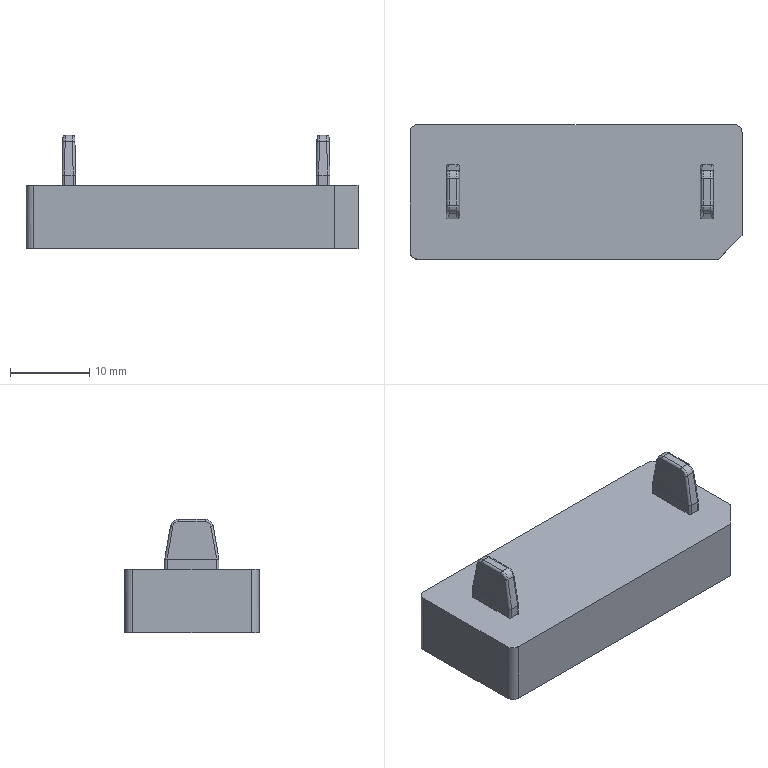NC program | PowerMill | posted by the shop | part box 42 x 17 x 14.346 mm
Lines 3506 to 4334 of 86217:
( TOOL ID   D10_1_1 )
( TOOL DIA. 10. TIP RAD 0 LENGTH 69.52 )
( Z = -.274 )
T3 M6
T4
G91 G28 Z0
G0 G90 G54
M08
S8500 M3
X0 Y0 M8
G43 Z11.796 H3
X-11.537 Y-11.817
Z.926
G1 Z-.274 F360
X-13.342 Y-6.86 F600
X-13.849 Y7.05
X-14.067 Y7.097
X-14.384 Y7.153
X-14.7 Y7.182
X-15.017 Y7.195
X-15.333 Y7.194
X-15.649 Y7.186
X-16.282 Y7.179
X-16.598 Y7.157
X-16.914 Y7.115
X-17.231 Y7.053
X-17.547 Y6.97
X-17.819 Y6.883
X-17.313 Y-7.01
G0 Z3.996
G1 X21.398 Y-11.505 F10000
G0 Z.926
G1 Z-.274 F360
X19.185 Y-6.717 F600
X17.985 Y7.118
X17.863 Y7.14
X17.547 Y7.175
X17.23 Y7.195
X16.914 Y7.199
X16.598 Y7.185
X15.965 Y7.184
X15.649 Y7.164
X15.332 Y7.128
X15.016 Y7.072
X14.699 Y6.996
X14.383 Y6.897
X14.067 Y6.779
X13.974 Y6.738
X15.172 Y-7.076
G0 Z11.796
X0 Y0
Z9.796
X31.66 Y.061
Z-5.35
G1 Z-6.55 F360
X26.385 F600
X22.805
Y-3.109
X22.798 Y-3.392
X22.769 Y-3.737
X22.733 Y-4.009
X22.683 Y-4.278
X22.62 Y-4.545
X22.524 Y-4.869
X22.441 Y-5.109
X22.346 Y-5.346
X22.241 Y-5.578
X22.124 Y-5.805
G2 X21.841 Y-6.277 I-5.278 J2.842
X21.512 Y-6.718 I-5.134 J3.488
G1 X21.346 Y-6.913
G2 X20.985 Y-7.279 I-4.426 J3.999
X20.554 Y-7.641 I-4.73 J5.201
X19.7 Y-8.174 I-3.44 J4.554
G1 X19.414 Y-8.312
X19.173 Y-8.411
X18.868 Y-8.518
X18.598 Y-8.599
X18.325 Y-8.666
X18.048 Y-8.718
X17.769 Y-8.756
G2 X17.124 Y-8.794 I-.663 J5.709
G1 X15.841 Y-8.791
X15.616 Y-8.778
X15.391 Y-8.756
X15.112 Y-8.718
X14.835 Y-8.666
X14.562 Y-8.599
G2 X13.987 Y-8.411 I1.929 J6.87
G1 X13.746 Y-8.312
G2 X13.232 Y-8.052 I2.536 J5.659
G1 X13.017 Y-7.925
G2 X12.591 Y-7.629 I3.181 J5.035
G1 X12.41 Y-7.485
G2 X11.99 Y-7.1 I3.923 J4.714
X11.319 Y-6.277 I4.33 J4.216
G1 X11.186 Y-6.068
X11.036 Y-5.805
X10.919 Y-5.578
G2 X10.617 Y-4.808 I5.201 J2.49
G1 X10.54 Y-4.545
X10.477 Y-4.278
X10.427 Y-4.009
X10.391 Y-3.737
X10.362 Y-3.392
X10.355 Y-3.109
Y3.148
X10.362 Y3.431
X10.391 Y3.776
X10.427 Y4.048
X10.477 Y4.318
X10.54 Y4.584
X10.636 Y4.908
X10.719 Y5.149
X10.814 Y5.385
X10.919 Y5.617
X11.036 Y5.844
G2 X11.319 Y6.316 I5.259 J-2.831
X11.648 Y6.757 I5.132 J-3.486
G1 X11.814 Y6.952
G2 X12.175 Y7.318 I4.415 J-3.988
X12.606 Y7.68 I4.7 J-5.165
X13.017 Y7.964 I3.646 J-4.838
G1 X13.28 Y8.118
X13.511 Y8.24
X13.746 Y8.351
X14.016 Y8.461
X14.233 Y8.538
G2 X14.835 Y8.705 I1.983 J-5.972
G1 X15.112 Y8.757
X15.391 Y8.795
G2 X16.036 Y8.834 I.667 J-5.782
G1 X17.233 Y8.832
G2 X17.9 Y8.777 I-.091 J-5.246
G1 X18.048 Y8.757
G2 X18.598 Y8.638 I-1.065 J-6.25
X19.173 Y8.45 I-1.914 J-6.822
X20.093 Y7.993 I-2.078 J-5.341
G1 X20.257 Y7.89
X20.554 Y7.68
X20.792 Y7.488
X20.985 Y7.318
X21.17 Y7.14
G2 X21.974 Y6.108 I-4.196 J-4.1
G1 X22.097 Y5.893
G2 X22.346 Y5.385 I-5.508 J-3.016
G1 X22.441 Y5.149
X22.543 Y4.848
X22.62 Y4.584
X22.683 Y4.318
X22.733 Y4.048
X22.769 Y3.776
X22.798 Y3.431
X22.805 Y3.148
Y.061
X26.385
G0 Z2.856
G1 X-31.66 Y.02 F10000
G0 Z-5.35
G1 Z-6.55 F360
X-26.385 F600
X-21.805
Y3.148
X-21.798 Y3.431
X-21.769 Y3.776
X-21.733 Y4.048
X-21.683 Y4.318
X-21.62 Y4.584
X-21.51 Y4.951
X-21.441 Y5.149
X-21.346 Y5.385
X-21.241 Y5.617
G2 X-20.841 Y6.316 I5.578 J-2.725
G1 X-20.699 Y6.518
X-20.512 Y6.757
X-20.346 Y6.952
X-20.17 Y7.14
G2 X-19.717 Y7.549 I4.101 J-4.072
G1 X-19.554 Y7.68
G2 X-18.946 Y8.08 I3.381 J-4.47
X-18.173 Y8.45 I2.795 J-4.851
X-17.598 Y8.638 I2.5 J-6.67
X-17.048 Y8.757 I1.632 J-6.207
G1 X-16.769 Y8.795
G2 X-16.124 Y8.834 I.668 J-5.798
G1 X-14.947 Y8.832
G2 X-14.271 Y8.779 I-.068 J-5.2
G1 X-14.112 Y8.757
X-13.835 Y8.705
G2 X-13.122 Y8.499 I-1.254 J-5.662
X-12.42 Y8.192 I-1.656 J-4.761
X-11.549 Y7.635 I-2.474 J-4.822
G1 X-11.359 Y7.48
X-11.175 Y7.318
X-10.99 Y7.14
X-10.814 Y6.952
G2 X-10.461 Y6.518 I-5.166 J-4.566
X-10.036 Y5.844 I-4.569 J-3.352
G1 X-9.919 Y5.617
G2 X-9.719 Y5.149 I-5.583 J-2.662
G1 X-9.617 Y4.848
X-9.54 Y4.584
X-9.477 Y4.318
X-9.427 Y4.048
X-9.385 Y3.713
X-9.362 Y3.431
X-9.355 Y3.148
Y.487
X.465 Y.636
X.514 Y-2.554
G2 X.474 Y-3.952 I-16.134 J-.244
G1 X.469 Y-4.025
G3 X.52 Y-4.08 I.051 J-.004
G1 X.54
G3 X.592 Y-4.025 I0 J.052
G1 X.57 Y-3.53
X.478 Y2.325
G2 X.529 Y3.956 I17.263 J.27
G1 X.535 Y4.032
G3 X.485 Y4.087 I-.051 J.004
G1 X.461
G3 X.408 Y4.031 I0 J-.053
G1 X.417 Y3.826
X.465 Y.636
X-4.521 Y.56
X-4.56 Y3.429
X-4.573 Y3.696
G3 X-5.417 Y7.309 I-10.448 J-.535
G1 X-5.709 Y7.986
G2 X-4.991 Y9.078 I.718 J.31
G1 X5.994 Y9.079
G2 X6.705 Y7.974 I0 J-.781
G1 X6.571 Y7.68
G3 X5.469 Y2.408 I11.158 J-5.085
G1 X5.558 Y-3.337
G3 X5.97 Y-6.021 I10.686 J.264
G1 X6.101 Y-6.446
G3 X6.445 Y-7.339 I9.337 J3.09
G1 X6.532 Y-7.535
X6.737 Y-7.95
G2 X6.047 Y-9.065 I-.69 J-.344
G1 X-5.017 Y-9.079
G2 X-5.725 Y-7.971 I-.001 J.78
G1 X-5.592 Y-7.683
X-5.332 Y-7.082
X-5.268 Y-6.921
G3 X-4.477 Y-2.647 I-10.334 J4.122
G1 X-4.521 Y.56
X-9.355 Y.487
Y-3.109
X-9.362 Y-3.392
G2 X-9.427 Y-4.009 I-7.113 J.434
G1 X-9.477 Y-4.278
G2 X-9.814 Y-5.346 I-5.909 J1.278
G1 X-9.919 Y-5.578
X-10.063 Y-5.854
X-10.186 Y-6.068
X-10.319 Y-6.277
X-10.461 Y-6.479
G2 X-10.99 Y-7.1 I-4.994 J3.717
G1 X-11.175 Y-7.279
X-11.41 Y-7.485
X-11.606 Y-7.641
X-11.808 Y-7.787
X-12.017 Y-7.925
X-12.227 Y-8.049
X-12.511 Y-8.201
G2 X-12.987 Y-8.411 I-2.772 J5.65
G1 X-13.292 Y-8.518
X-13.562 Y-8.599
X-13.835 Y-8.666
X-14.112 Y-8.718
X-14.391 Y-8.756
G2 X-15.036 Y-8.794 I-.659 J5.646
G1 X-16.124
X-16.319 Y-8.791
G2 X-17.325 Y-8.666 I.251 J6.13
X-18.414 Y-8.312 I1.32 J5.917
X-19.352 Y-7.787 I2.453 J5.49
X-19.792 Y-7.449 I3.506 J5.014
G1 X-19.985 Y-7.279
X-20.17 Y-7.1
X-20.346 Y-6.913
G2 X-20.699 Y-6.479 I5.161 J4.562
X-21.124 Y-5.805 I4.594 J3.368
G1 X-21.241 Y-5.578
G2 X-21.441 Y-5.109 I5.678 J2.703
G1 X-21.543 Y-4.808
X-21.62 Y-4.545
X-21.683 Y-4.278
X-21.733 Y-4.009
X-21.769 Y-3.737
G2 X-21.805 Y-3.109 I6.227 J.676
G1 Y.02
X-26.385
G0 Z9.796
X0 Y0
X26.008 Y-14.747
Z-13.25
G1 Z-14.45 F360
G3 X22.473 Y-11.211 I-1.768 J1.768 F600
G1 X21.614 Y-12.07
X21.613 Y-12.071
X21.395 Y-12.279
X21.394 Y-12.28
X21.392 Y-12.281
X21.267 Y-12.39
X21.266 Y-12.391
X21.265 Y-12.392
X21.074 Y-12.545
X21.072 Y-12.546
X21.07 Y-12.547
X20.842 Y-12.711
X20.84 Y-12.712
X20.839 Y-12.713
X20.752 Y-12.77
X20.75 Y-12.771
X20.748 Y-12.772
X20.432 Y-12.96
X20.43 Y-12.961
X20.429 Y-12.962
X20.293 Y-13.033
X20.292
X20.291 Y-13.034
X20.11 Y-13.121
X20.108 Y-13.122
X20.106 Y-13.123
X19.79 Y-13.254
X19.787 Y-13.255
X19.785 Y-13.256
X19.499 Y-13.354
X19.496 Y-13.355
X19.494
X19.148 Y-13.449
X19.145
X19.142 Y-13.45
X18.826 Y-13.512
X18.824 Y-13.513
X18.821
X18.505 Y-13.555
X18.502
X18.5
X18.184 Y-13.577
X18.181
X18.179
X17.863 Y-13.58
X17.862
X-20.075 Y-13.579
X-20.077
X-20.078
X-20.394 Y-13.567
X-20.397
X-20.399
X-20.715 Y-13.538
X-20.717 Y-13.537
X-20.719
X-21.035 Y-13.491
X-21.037
X-21.039 Y-13.49
X-21.356 Y-13.427
X-21.358 Y-13.426
X-21.36
X-21.636 Y-13.356
X-21.638 Y-13.355
X-21.64 Y-13.354
X-21.996 Y-13.243
X-21.998 Y-13.242
X-22.001 Y-13.241
X-22.317 Y-13.121
X-22.319 Y-13.12
X-22.321
X-22.637 Y-12.978
X-22.639 Y-12.977
X-22.641 Y-12.976
X-22.957 Y-12.812
X-22.959 Y-12.811
X-22.961 Y-12.81
X-23.125 Y-12.715
X-23.127 Y-12.714
X-23.128
X-23.279 Y-12.62
X-23.28 Y-12.619
X-23.282 Y-12.618
X-23.598 Y-12.401
X-23.6 Y-12.399
X-23.602 Y-12.398
X-23.919 Y-12.149
X-23.92 Y-12.148
X-23.921 Y-12.147
X-24.005 Y-12.074
X-24.006 Y-12.073
X-24.008 Y-12.072
X-24.239 Y-11.858
X-24.241 Y-11.857
X-24.242 Y-11.856
X-24.344 Y-11.754
X-24.345 Y-11.753
X-24.346 Y-11.752
X-24.56 Y-11.522
X-24.561 Y-11.52
X-24.562 Y-11.519
X-24.636 Y-11.433
X-24.637 Y-11.432
Y-11.431
X-24.88 Y-11.126
X-24.882 Y-11.124
X-24.883 Y-11.122
X-25.11 Y-10.794
X-25.111 Y-10.793
X-25.112 Y-10.791
X-25.201 Y-10.648
X-25.202 Y-10.647
X-25.203 Y-10.646
X-25.303 Y-10.473
X-25.304 Y-10.471
X-25.305 Y-10.47
X-25.47 Y-10.154
X-25.471 Y-10.152
X-25.472 Y-10.149
X-25.614 Y-9.833
X-25.615 Y-9.831
X-25.616 Y-9.829
X-25.737 Y-9.513
X-25.738 Y-9.511
X-25.739 Y-9.509
X-25.84 Y-9.193
Y-9.19
X-25.841 Y-9.188
X-25.923 Y-8.872
X-25.924 Y-8.87
Y-8.868
X-25.988 Y-8.552
Y-8.55
Y-8.548
X-26.036 Y-8.232
Y-8.229
Y-8.227
X-26.065 Y-7.911
Y-7.909
X-26.066 Y-7.907
X-26.079 Y-7.591
Y-7.589
Y-7.587
Y7.587
Y7.589
Y7.591
X-26.066 Y7.907
Y7.909
Y7.911
X-26.036 Y8.227
Y8.229
Y8.231
X-25.989 Y8.548
Y8.55
X-25.988 Y8.552
X-25.924 Y8.868
Y8.87
X-25.923 Y8.872
X-25.843 Y9.179
Y9.182
X-25.842 Y9.184
X-25.738 Y9.509
Y9.511
X-25.737 Y9.513
X-25.616 Y9.829
X-25.615 Y9.831
X-25.614 Y9.833
X-25.472 Y10.149
X-25.471 Y10.152
X-25.47 Y10.154
X-25.305 Y10.47
X-25.304 Y10.471
X-25.303 Y10.473
X-25.203 Y10.646
X-25.202 Y10.647
X-25.201 Y10.648
X-25.112 Y10.791
X-25.111 Y10.793
X-25.11 Y10.794
X-24.892 Y11.111
X-24.89 Y11.113
X-24.889 Y11.115
X-24.638 Y11.431
X-24.637 Y11.432
X-24.636 Y11.434
X-24.562 Y11.519
X-24.561 Y11.521
X-24.56 Y11.522
X-24.346 Y11.752
X-24.345 Y11.753
X-24.344 Y11.754
X-24.242 Y11.856
X-24.241 Y11.857
X-24.239 Y11.858
X-24.007 Y12.072
X-24.006 Y12.073
X-24.005 Y12.074
X-23.921 Y12.146
X-23.92 Y12.147
X-23.919 Y12.148
X-23.61 Y12.392
X-23.608 Y12.394
X-23.605 Y12.396
X-23.282 Y12.618
X-23.28 Y12.619
X-23.279 Y12.62
X-23.128 Y12.714
X-23.127
X-23.125 Y12.715
X-22.961 Y12.81
X-22.959 Y12.811
X-22.957 Y12.812
X-22.641 Y12.976
X-22.639 Y12.977
X-22.637 Y12.978
X-22.321 Y13.12
X-22.319
X-22.317 Y13.121
X-22.001 Y13.241
X-21.998 Y13.242
X-21.996 Y13.243
X-21.68 Y13.343
X-21.678 Y13.344
X-21.676
X-21.36 Y13.426
X-21.358
X-21.355 Y13.427
X-21.039 Y13.49
X-21.037
X-21.035
X-20.719 Y13.537
X-20.717
X-20.715 Y13.538
X-20.399 Y13.566
X-20.397
X-20.395
X-20.079 Y13.579
X-20.077
X-20.075
X-.316
X20.075
X20.077
X20.078
X20.394 Y13.567
X20.397
X20.399
X20.715 Y13.538
X20.717 Y13.537
X20.719
X21.035 Y13.491
X21.037
X21.039 Y13.49
X21.356 Y13.427
X21.358 Y13.426
X21.36
X21.636 Y13.356
X21.638 Y13.355
X21.64 Y13.354
X21.996 Y13.243
X21.998 Y13.242
X22.001 Y13.241
X22.317 Y13.121
X22.319 Y13.12
X22.321
X22.637 Y12.978
X22.639 Y12.977
X22.641 Y12.976
X22.957 Y12.812
X22.959 Y12.811
X22.961 Y12.81
X23.125 Y12.715
X23.127 Y12.714
X23.128
X23.279 Y12.62
X23.28 Y12.619
X23.282 Y12.618
X23.598 Y12.401
X23.6 Y12.399
X23.602 Y12.398
X23.919 Y12.149
X23.92 Y12.148
X23.921 Y12.147
X24.005 Y12.074
X24.006 Y12.073
X24.008 Y12.072
X24.239 Y11.858
X24.241 Y11.857
X24.242 Y11.856
X24.344 Y11.754
X24.345 Y11.753
X24.346 Y11.752
X24.56 Y11.522
X24.561 Y11.52
X24.562 Y11.519
X24.636 Y11.433
X24.637 Y11.432
Y11.431
X24.88 Y11.126
X24.882 Y11.124
X24.883 Y11.122
X25.11 Y10.794
X25.111 Y10.793
X25.112 Y10.791
X25.201 Y10.648
X25.202 Y10.647
X25.203 Y10.646
X25.303 Y10.473
X25.304 Y10.471
X25.305 Y10.47
X25.47 Y10.154
X25.471 Y10.152
X25.472 Y10.149
X25.614 Y9.833
X25.615 Y9.831
X25.616 Y9.829
X25.737 Y9.513
X25.738 Y9.511
X25.739 Y9.509
X25.84 Y9.193
Y9.19
X25.841 Y9.188
X25.923 Y8.872
X25.924 Y8.87
Y8.868
X25.988 Y8.552
Y8.55
Y8.548
X26.036 Y8.232
Y8.229
Y8.227
X26.065 Y7.911
Y7.909
X26.066 Y7.907
X26.079 Y7.591
Y7.589
Y7.588
X26.08 Y-5.374
Y-5.375
X26.076 Y-5.692
Y-5.694
Y-5.696
X26.054 Y-6.012
Y-6.015
Y-6.017
X26.011 Y-6.334
Y-6.336
X26.01 Y-6.339
X25.947 Y-6.655
X25.946 Y-6.657
Y-6.66
X25.861 Y-6.976
X25.86 Y-6.979
X25.859 Y-6.981
X25.751 Y-7.297
Y-7.3
X25.75 Y-7.302
X25.617 Y-7.618
X25.616 Y-7.62
X25.615 Y-7.622
X25.522 Y-7.815
X25.521 Y-7.817
X25.52 Y-7.818
X25.455 Y-7.941
X25.454 Y-7.943
X25.453 Y-7.945
X25.264 Y-8.261
X25.263 Y-8.262
X25.262 Y-8.264
X25.2 Y-8.357
X25.199 Y-8.359
X25.198 Y-8.36
X25.038 Y-8.583
X25.036 Y-8.584
X25.035 Y-8.586
X24.88 Y-8.779
X24.879 Y-8.781
X24.878 Y-8.782
X24.77 Y-8.905
X24.769 Y-8.906
X24.768 Y-8.907
X24.559 Y-9.125
X24.558 Y-9.126
X22.473 Y-11.211
G3 X26.008 Y-14.747 I1.768 J-1.768
G1 X25.957 Y-14.685
G3 X22.422 Y-11.149 I-1.768 J1.768
G1 X21.558 Y-12.014
X21.34 Y-12.221
X21.215 Y-12.33
X21.024 Y-12.482
X20.795 Y-12.646
X20.708 Y-12.703
X20.391 Y-12.891
X20.256 Y-12.962
X20.075 Y-13.049
X19.759 Y-13.18
X19.473 Y-13.278
X19.127 Y-13.371
X18.811 Y-13.434
X18.495 Y-13.475
X18.178 Y-13.497
X17.862 Y-13.5
X-19.443
X-20.075 Y-13.499
X-20.391 Y-13.487
X-20.708 Y-13.458
X-21.024 Y-13.412
X-21.34 Y-13.348
X-21.616 Y-13.278
X-21.972 Y-13.167
X-22.288 Y-13.047
X-22.604 Y-12.905
X-22.921 Y-12.741
X-23.085 Y-12.646
X-23.237 Y-12.552
X-23.553 Y-12.335
X-23.869 Y-12.086
X-23.953 Y-12.014
X-24.185 Y-11.799
X-24.287 Y-11.697
X-24.501 Y-11.467
X-24.575 Y-11.381
X-24.817 Y-11.077
X-25.044 Y-10.749
X-25.134 Y-10.606
X-25.234 Y-10.433
X-25.399 Y-10.117
X-25.541 Y-9.801
X-25.662 Y-9.484
X-25.763 Y-9.168
X-25.846 Y-8.852
X-25.909 Y-8.536
X-25.957 Y-8.22
X-25.986 Y-7.904
X-25.999 Y-7.587
X-26. Y-7.271
Y7.271
X-25.999 Y7.587
X-25.986 Y7.904
X-25.957 Y8.22
X-25.91 Y8.536
X-25.846 Y8.852
X-25.766 Y9.159
X-25.662 Y9.484
X-25.541 Y9.801
X-25.399 Y10.117
X-25.234 Y10.433
X-25.134 Y10.606
X-25.044 Y10.749
X-24.826 Y11.065
X-24.576 Y11.381
X-24.501 Y11.467
X-24.287 Y11.697
X-24.185 Y11.799
X-23.953 Y12.014
X-23.869 Y12.085
X-23.56 Y12.33
X-23.237 Y12.552
X-23.085 Y12.646
X-22.921 Y12.741
X-22.604 Y12.905
X-22.288 Y13.047
X-21.972 Y13.167
X-21.656 Y13.267
X-21.34 Y13.348
X-21.024 Y13.411
X-20.708 Y13.458
X-20.391 Y13.486
X-20.075 Y13.499
X-19.759 Y13.5
X-.316
X19.127
X20.075 Y13.499
X20.391 Y13.487
X20.708 Y13.458
X21.024 Y13.412
X21.34 Y13.348
X21.616 Y13.278
X21.972 Y13.167
X22.288 Y13.047
X22.604 Y12.905
X22.921 Y12.741
X23.085 Y12.646
X23.237 Y12.552
X23.553 Y12.335
X23.869 Y12.086
X23.953 Y12.014
X24.185 Y11.799
X24.287 Y11.697
X24.501 Y11.467
X24.575 Y11.381
X24.817 Y11.077
X25.044 Y10.749
X25.134 Y10.606
X25.234 Y10.433
X25.399 Y10.117
X25.541 Y9.801
X25.662 Y9.484
X25.763 Y9.168
X25.846 Y8.852
X25.909 Y8.536
X25.957 Y8.22
X25.986 Y7.904
X25.999 Y7.587
X26. Y7.271
Y-5.374
X25.996 Y-5.691
X25.974 Y-6.007
X25.932 Y-6.323
X25.869 Y-6.639
X25.784 Y-6.955
X25.676 Y-7.271
X25.543 Y-7.587
X25.45 Y-7.78
X25.384 Y-7.904
X25.196 Y-8.22
X25.134 Y-8.313
X24.973 Y-8.536
X24.817 Y-8.729
X24.71 Y-8.852
X24.501 Y-9.07
X22.422 Y-11.149
G3 X25.957 Y-14.685 I1.768 J-1.768
G0 Z9.796
Z10.796
X0 Y0
M9
M5
M01